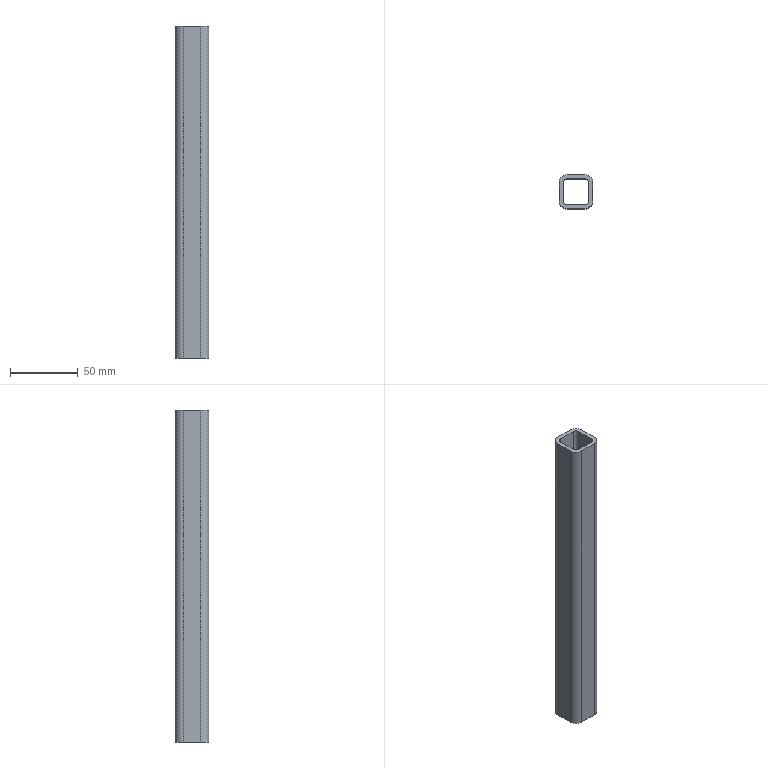Part | STEP file | ISO 10799-2 25x25x3 1784906820939 | 1 solid | 18 faces | box 25 x 25 x 245 mm | volume 59002 mm3 | plane 10 | cylinder 8 | commonest cylinder face diameters 6 x4 12 x4
STEP:
#1=CARTESIAN_POINT('',(-6.5,-9.5,245.));
#2=VERTEX_POINT('',#1);
#3=CARTESIAN_POINT('',(6.5,-9.5,245.));
#4=VERTEX_POINT('',#3);
#5=CARTESIAN_POINT('',(3.25,-9.5,245.));
#6=DIRECTION('',(1.,0.,0.));
#7=VECTOR('',#6,10.);
#8=LINE('',#5,#7);
#9=EDGE_CURVE('',#2,#4,#8,.T.);
#10=ORIENTED_EDGE('',*,*,#9,.T.);
#11=CARTESIAN_POINT('',(6.5,-9.5,0.));
#12=VERTEX_POINT('',#11);
#13=CARTESIAN_POINT('',(6.5,-9.5,0.));
#14=DIRECTION('',(0.,0.,1.));
#15=VECTOR('',#14,10.);
#16=LINE('',#13,#15);
#17=EDGE_CURVE('',#12,#4,#16,.T.);
#18=ORIENTED_EDGE('',*,*,#17,.F.);
#19=CARTESIAN_POINT('',(-6.5,-9.5,0.));
#20=VERTEX_POINT('',#19);
#21=CARTESIAN_POINT('',(3.25,-9.5,0.));
#22=DIRECTION('',(1.,0.,0.));
#23=VECTOR('',#22,10.);
#24=LINE('',#21,#23);
#25=EDGE_CURVE('',#20,#12,#24,.T.);
#26=ORIENTED_EDGE('',*,*,#25,.F.);
#27=CARTESIAN_POINT('',(-6.5,-9.5,0.));
#28=DIRECTION('',(0.,0.,1.));
#29=VECTOR('',#28,10.);
#30=LINE('',#27,#29);
#31=EDGE_CURVE('',#20,#2,#30,.T.);
#32=ORIENTED_EDGE('',*,*,#31,.T.);
#33=EDGE_LOOP('',(#10,#18,#26,#32));
#34=FACE_OUTER_BOUND('',#33,.T.);
#35=CARTESIAN_POINT('',(6.5,-9.5,0.));
#36=DIRECTION('',(0.,-1.,0.));
#37=DIRECTION('',(0.,0.,-1.));
#38=AXIS2_PLACEMENT_3D('',#35,#36,#37);
#39=PLANE('',#38);
#40=ADVANCED_FACE('',(#34),#39,.F.);
#41=CARTESIAN_POINT('',(9.5,-6.5,245.));
#42=VERTEX_POINT('',#41);
#43=CARTESIAN_POINT('',(6.5,-6.5,245.));
#44=DIRECTION('',(0.,0.,1.));
#45=DIRECTION('',(0.,1.,0.));
#46=AXIS2_PLACEMENT_3D('',#43,#44,#45);
#47=CIRCLE('',#46,3.);
#48=EDGE_CURVE('',#4,#42,#47,.T.);
#49=ORIENTED_EDGE('',*,*,#48,.T.);
#50=CARTESIAN_POINT('',(9.5,-6.5,0.));
#51=VERTEX_POINT('',#50);
#52=CARTESIAN_POINT('',(9.5,-6.5,0.));
#53=DIRECTION('',(0.,0.,1.));
#54=VECTOR('',#53,10.);
#55=LINE('',#52,#54);
#56=EDGE_CURVE('',#51,#42,#55,.T.);
#57=ORIENTED_EDGE('',*,*,#56,.F.);
#58=CARTESIAN_POINT('',(6.5,-6.5,0.));
#59=DIRECTION('',(0.,0.,1.));
#60=DIRECTION('',(0.,1.,0.));
#61=AXIS2_PLACEMENT_3D('',#58,#59,#60);
#62=CIRCLE('',#61,3.);
#63=EDGE_CURVE('',#12,#51,#62,.T.);
#64=ORIENTED_EDGE('',*,*,#63,.F.);
#65=ORIENTED_EDGE('',*,*,#17,.T.);
#66=EDGE_LOOP('',(#49,#57,#64,#65));
#67=FACE_OUTER_BOUND('',#66,.T.);
#68=CARTESIAN_POINT('',(6.5,-6.5,0.));
#69=DIRECTION('',(0.,0.,1.));
#70=DIRECTION('',(0.,1.,0.));
#71=AXIS2_PLACEMENT_3D('',#68,#69,#70);
#72=CYLINDRICAL_SURFACE('',#71,3.);
#73=ADVANCED_FACE('',(#67),#72,.F.);
#74=CARTESIAN_POINT('',(9.5,6.5,245.));
#75=VERTEX_POINT('',#74);
#76=CARTESIAN_POINT('',(9.5,3.25,245.));
#77=DIRECTION('',(0.,1.,0.));
#78=VECTOR('',#77,10.);
#79=LINE('',#76,#78);
#80=EDGE_CURVE('',#42,#75,#79,.T.);
#81=ORIENTED_EDGE('',*,*,#80,.T.);
#82=CARTESIAN_POINT('',(9.5,6.5,0.));
#83=VERTEX_POINT('',#82);
#84=CARTESIAN_POINT('',(9.5,6.5,0.));
#85=DIRECTION('',(0.,0.,1.));
#86=VECTOR('',#85,10.);
#87=LINE('',#84,#86);
#88=EDGE_CURVE('',#83,#75,#87,.T.);
#89=ORIENTED_EDGE('',*,*,#88,.F.);
#90=CARTESIAN_POINT('',(9.5,3.25,0.));
#91=DIRECTION('',(0.,1.,0.));
#92=VECTOR('',#91,10.);
#93=LINE('',#90,#92);
#94=EDGE_CURVE('',#51,#83,#93,.T.);
#95=ORIENTED_EDGE('',*,*,#94,.F.);
#96=ORIENTED_EDGE('',*,*,#56,.T.);
#97=EDGE_LOOP('',(#81,#89,#95,#96));
#98=FACE_OUTER_BOUND('',#97,.T.);
#99=CARTESIAN_POINT('',(9.5,6.5,0.));
#100=DIRECTION('',(1.,0.,0.));
#101=DIRECTION('',(0.,0.,-1.));
#102=AXIS2_PLACEMENT_3D('',#99,#100,#101);
#103=PLANE('',#102);
#104=ADVANCED_FACE('',(#98),#103,.F.);
#105=CARTESIAN_POINT('',(6.5,9.5,245.));
#106=VERTEX_POINT('',#105);
#107=CARTESIAN_POINT('',(6.5,6.5,245.));
#108=DIRECTION('',(0.,0.,1.));
#109=DIRECTION('',(-1.,0.,0.));
#110=AXIS2_PLACEMENT_3D('',#107,#108,#109);
#111=CIRCLE('',#110,3.);
#112=EDGE_CURVE('',#75,#106,#111,.T.);
#113=ORIENTED_EDGE('',*,*,#112,.T.);
#114=CARTESIAN_POINT('',(6.5,9.5,0.));
#115=VERTEX_POINT('',#114);
#116=CARTESIAN_POINT('',(6.5,9.5,0.));
#117=DIRECTION('',(0.,0.,1.));
#118=VECTOR('',#117,10.);
#119=LINE('',#116,#118);
#120=EDGE_CURVE('',#115,#106,#119,.T.);
#121=ORIENTED_EDGE('',*,*,#120,.F.);
#122=CARTESIAN_POINT('',(6.5,6.5,0.));
#123=DIRECTION('',(0.,0.,1.));
#124=DIRECTION('',(-1.,0.,0.));
#125=AXIS2_PLACEMENT_3D('',#122,#123,#124);
#126=CIRCLE('',#125,3.);
#127=EDGE_CURVE('',#83,#115,#126,.T.);
#128=ORIENTED_EDGE('',*,*,#127,.F.);
#129=ORIENTED_EDGE('',*,*,#88,.T.);
#130=EDGE_LOOP('',(#113,#121,#128,#129));
#131=FACE_OUTER_BOUND('',#130,.T.);
#132=CARTESIAN_POINT('',(6.5,6.5,0.));
#133=DIRECTION('',(0.,0.,1.));
#134=DIRECTION('',(-1.,0.,0.));
#135=AXIS2_PLACEMENT_3D('',#132,#133,#134);
#136=CYLINDRICAL_SURFACE('',#135,3.);
#137=ADVANCED_FACE('',(#131),#136,.F.);
#138=CARTESIAN_POINT('',(12.5,6.5,245.));
#139=VERTEX_POINT('',#138);
#140=CARTESIAN_POINT('',(12.5,-6.5,245.));
#141=VERTEX_POINT('',#140);
#142=CARTESIAN_POINT('',(12.5,3.25,245.));
#143=DIRECTION('',(0.,-1.,0.));
#144=VECTOR('',#143,10.);
#145=LINE('',#142,#144);
#146=EDGE_CURVE('',#139,#141,#145,.T.);
#147=ORIENTED_EDGE('',*,*,#146,.T.);
#148=CARTESIAN_POINT('',(12.5,-6.5,0.));
#149=VERTEX_POINT('',#148);
#150=CARTESIAN_POINT('',(12.5,-6.5,0.));
#151=DIRECTION('',(0.,0.,1.));
#152=VECTOR('',#151,10.);
#153=LINE('',#150,#152);
#154=EDGE_CURVE('',#149,#141,#153,.T.);
#155=ORIENTED_EDGE('',*,*,#154,.F.);
#156=CARTESIAN_POINT('',(12.5,6.5,0.));
#157=VERTEX_POINT('',#156);
#158=CARTESIAN_POINT('',(12.5,3.25,0.));
#159=DIRECTION('',(0.,-1.,0.));
#160=VECTOR('',#159,10.);
#161=LINE('',#158,#160);
#162=EDGE_CURVE('',#157,#149,#161,.T.);
#163=ORIENTED_EDGE('',*,*,#162,.F.);
#164=CARTESIAN_POINT('',(12.5,6.5,0.));
#165=DIRECTION('',(0.,0.,1.));
#166=VECTOR('',#165,10.);
#167=LINE('',#164,#166);
#168=EDGE_CURVE('',#157,#139,#167,.T.);
#169=ORIENTED_EDGE('',*,*,#168,.T.);
#170=EDGE_LOOP('',(#147,#155,#163,#169));
#171=FACE_OUTER_BOUND('',#170,.T.);
#172=CARTESIAN_POINT('',(12.5,6.5,0.));
#173=DIRECTION('',(1.,0.,0.));
#174=DIRECTION('',(0.,0.,-1.));
#175=AXIS2_PLACEMENT_3D('',#172,#173,#174);
#176=PLANE('',#175);
#177=ADVANCED_FACE('',(#171),#176,.T.);
#178=CARTESIAN_POINT('',(6.5,-12.5,245.));
#179=VERTEX_POINT('',#178);
#180=CARTESIAN_POINT('',(6.5,-6.5,245.));
#181=DIRECTION('',(0.,0.,-1.));
#182=DIRECTION('',(0.,1.,0.));
#183=AXIS2_PLACEMENT_3D('',#180,#181,#182);
#184=CIRCLE('',#183,6.);
#185=EDGE_CURVE('',#141,#179,#184,.T.);
#186=ORIENTED_EDGE('',*,*,#185,.T.);
#187=CARTESIAN_POINT('',(6.5,-12.5,0.));
#188=VERTEX_POINT('',#187);
#189=CARTESIAN_POINT('',(6.5,-12.5,0.));
#190=DIRECTION('',(0.,0.,1.));
#191=VECTOR('',#190,10.);
#192=LINE('',#189,#191);
#193=EDGE_CURVE('',#188,#179,#192,.T.);
#194=ORIENTED_EDGE('',*,*,#193,.F.);
#195=CARTESIAN_POINT('',(6.5,-6.5,0.));
#196=DIRECTION('',(0.,0.,-1.));
#197=DIRECTION('',(0.,1.,0.));
#198=AXIS2_PLACEMENT_3D('',#195,#196,#197);
#199=CIRCLE('',#198,6.);
#200=EDGE_CURVE('',#149,#188,#199,.T.);
#201=ORIENTED_EDGE('',*,*,#200,.F.);
#202=ORIENTED_EDGE('',*,*,#154,.T.);
#203=EDGE_LOOP('',(#186,#194,#201,#202));
#204=FACE_OUTER_BOUND('',#203,.T.);
#205=CARTESIAN_POINT('',(6.5,-6.5,0.));
#206=DIRECTION('',(0.,0.,1.));
#207=DIRECTION('',(0.,1.,0.));
#208=AXIS2_PLACEMENT_3D('',#205,#206,#207);
#209=CYLINDRICAL_SURFACE('',#208,6.);
#210=ADVANCED_FACE('',(#204),#209,.T.);
#211=CARTESIAN_POINT('',(-6.5,-12.5,245.));
#212=VERTEX_POINT('',#211);
#213=CARTESIAN_POINT('',(3.25,-12.5,245.));
#214=DIRECTION('',(-1.,0.,0.));
#215=VECTOR('',#214,10.);
#216=LINE('',#213,#215);
#217=EDGE_CURVE('',#179,#212,#216,.T.);
#218=ORIENTED_EDGE('',*,*,#217,.T.);
#219=CARTESIAN_POINT('',(-6.5,-12.5,0.));
#220=VERTEX_POINT('',#219);
#221=CARTESIAN_POINT('',(-6.5,-12.5,0.));
#222=DIRECTION('',(0.,0.,1.));
#223=VECTOR('',#222,10.);
#224=LINE('',#221,#223);
#225=EDGE_CURVE('',#220,#212,#224,.T.);
#226=ORIENTED_EDGE('',*,*,#225,.F.);
#227=CARTESIAN_POINT('',(3.25,-12.5,0.));
#228=DIRECTION('',(-1.,0.,0.));
#229=VECTOR('',#228,10.);
#230=LINE('',#227,#229);
#231=EDGE_CURVE('',#188,#220,#230,.T.);
#232=ORIENTED_EDGE('',*,*,#231,.F.);
#233=ORIENTED_EDGE('',*,*,#193,.T.);
#234=EDGE_LOOP('',(#218,#226,#232,#233));
#235=FACE_OUTER_BOUND('',#234,.T.);
#236=CARTESIAN_POINT('',(6.5,-12.5,0.));
#237=DIRECTION('',(0.,-1.,0.));
#238=DIRECTION('',(0.,0.,-1.));
#239=AXIS2_PLACEMENT_3D('',#236,#237,#238);
#240=PLANE('',#239);
#241=ADVANCED_FACE('',(#235),#240,.T.);
#242=CARTESIAN_POINT('',(-12.5,-6.5,245.));
#243=VERTEX_POINT('',#242);
#244=CARTESIAN_POINT('',(-6.5,-6.5,245.));
#245=DIRECTION('',(0.,0.,-1.));
#246=DIRECTION('',(1.,0.,0.));
#247=AXIS2_PLACEMENT_3D('',#244,#245,#246);
#248=CIRCLE('',#247,6.);
#249=EDGE_CURVE('',#212,#243,#248,.T.);
#250=ORIENTED_EDGE('',*,*,#249,.T.);
#251=CARTESIAN_POINT('',(-12.5,-6.5,0.));
#252=VERTEX_POINT('',#251);
#253=CARTESIAN_POINT('',(-12.5,-6.5,0.));
#254=DIRECTION('',(0.,0.,1.));
#255=VECTOR('',#254,10.);
#256=LINE('',#253,#255);
#257=EDGE_CURVE('',#252,#243,#256,.T.);
#258=ORIENTED_EDGE('',*,*,#257,.F.);
#259=CARTESIAN_POINT('',(-6.5,-6.5,0.));
#260=DIRECTION('',(0.,0.,-1.));
#261=DIRECTION('',(1.,0.,0.));
#262=AXIS2_PLACEMENT_3D('',#259,#260,#261);
#263=CIRCLE('',#262,6.);
#264=EDGE_CURVE('',#220,#252,#263,.T.);
#265=ORIENTED_EDGE('',*,*,#264,.F.);
#266=ORIENTED_EDGE('',*,*,#225,.T.);
#267=EDGE_LOOP('',(#250,#258,#265,#266));
#268=FACE_OUTER_BOUND('',#267,.T.);
#269=CARTESIAN_POINT('',(-6.5,-6.5,0.));
#270=DIRECTION('',(0.,0.,1.));
#271=DIRECTION('',(1.,0.,0.));
#272=AXIS2_PLACEMENT_3D('',#269,#270,#271);
#273=CYLINDRICAL_SURFACE('',#272,6.);
#274=ADVANCED_FACE('',(#268),#273,.T.);
#275=CARTESIAN_POINT('',(-6.5,9.5,245.));
#276=VERTEX_POINT('',#275);
#277=CARTESIAN_POINT('',(-3.25,9.5,245.));
#278=DIRECTION('',(-1.,0.,0.));
#279=VECTOR('',#278,10.);
#280=LINE('',#277,#279);
#281=EDGE_CURVE('',#106,#276,#280,.T.);
#282=ORIENTED_EDGE('',*,*,#281,.T.);
#283=CARTESIAN_POINT('',(-6.5,9.5,0.));
#284=VERTEX_POINT('',#283);
#285=CARTESIAN_POINT('',(-6.5,9.5,0.));
#286=DIRECTION('',(0.,0.,1.));
#287=VECTOR('',#286,10.);
#288=LINE('',#285,#287);
#289=EDGE_CURVE('',#284,#276,#288,.T.);
#290=ORIENTED_EDGE('',*,*,#289,.F.);
#291=CARTESIAN_POINT('',(-3.25,9.5,0.));
#292=DIRECTION('',(-1.,0.,0.));
#293=VECTOR('',#292,10.);
#294=LINE('',#291,#293);
#295=EDGE_CURVE('',#115,#284,#294,.T.);
#296=ORIENTED_EDGE('',*,*,#295,.F.);
#297=ORIENTED_EDGE('',*,*,#120,.T.);
#298=EDGE_LOOP('',(#282,#290,#296,#297));
#299=FACE_OUTER_BOUND('',#298,.T.);
#300=CARTESIAN_POINT('',(-6.5,9.5,0.));
#301=DIRECTION('',(0.,1.,0.));
#302=DIRECTION('',(0.,0.,1.));
#303=AXIS2_PLACEMENT_3D('',#300,#301,#302);
#304=PLANE('',#303);
#305=ADVANCED_FACE('',(#299),#304,.F.);
#306=CARTESIAN_POINT('',(-9.5,-6.5,245.));
#307=VERTEX_POINT('',#306);
#308=CARTESIAN_POINT('',(-6.5,-6.5,245.));
#309=DIRECTION('',(0.,0.,1.));
#310=DIRECTION('',(1.,0.,0.));
#311=AXIS2_PLACEMENT_3D('',#308,#309,#310);
#312=CIRCLE('',#311,3.);
#313=EDGE_CURVE('',#307,#2,#312,.T.);
#314=ORIENTED_EDGE('',*,*,#313,.T.);
#315=ORIENTED_EDGE('',*,*,#31,.F.);
#316=CARTESIAN_POINT('',(-9.5,-6.5,0.));
#317=VERTEX_POINT('',#316);
#318=CARTESIAN_POINT('',(-6.5,-6.5,0.));
#319=DIRECTION('',(0.,0.,1.));
#320=DIRECTION('',(1.,0.,0.));
#321=AXIS2_PLACEMENT_3D('',#318,#319,#320);
#322=CIRCLE('',#321,3.);
#323=EDGE_CURVE('',#317,#20,#322,.T.);
#324=ORIENTED_EDGE('',*,*,#323,.F.);
#325=CARTESIAN_POINT('',(-9.5,-6.5,0.));
#326=DIRECTION('',(0.,0.,1.));
#327=VECTOR('',#326,10.);
#328=LINE('',#325,#327);
#329=EDGE_CURVE('',#317,#307,#328,.T.);
#330=ORIENTED_EDGE('',*,*,#329,.T.);
#331=EDGE_LOOP('',(#314,#315,#324,#330));
#332=FACE_OUTER_BOUND('',#331,.T.);
#333=CARTESIAN_POINT('',(-6.5,-6.5,0.));
#334=DIRECTION('',(0.,0.,1.));
#335=DIRECTION('',(1.,0.,0.));
#336=AXIS2_PLACEMENT_3D('',#333,#334,#335);
#337=CYLINDRICAL_SURFACE('',#336,3.);
#338=ADVANCED_FACE('',(#332),#337,.F.);
#339=CARTESIAN_POINT('',(-9.5,6.5,245.));
#340=VERTEX_POINT('',#339);
#341=CARTESIAN_POINT('',(-9.5,-3.25,245.));
#342=DIRECTION('',(0.,-1.,0.));
#343=VECTOR('',#342,10.);
#344=LINE('',#341,#343);
#345=EDGE_CURVE('',#340,#307,#344,.T.);
#346=ORIENTED_EDGE('',*,*,#345,.T.);
#347=ORIENTED_EDGE('',*,*,#329,.F.);
#348=CARTESIAN_POINT('',(-9.5,6.5,0.));
#349=VERTEX_POINT('',#348);
#350=CARTESIAN_POINT('',(-9.5,-3.25,0.));
#351=DIRECTION('',(0.,-1.,0.));
#352=VECTOR('',#351,10.);
#353=LINE('',#350,#352);
#354=EDGE_CURVE('',#349,#317,#353,.T.);
#355=ORIENTED_EDGE('',*,*,#354,.F.);
#356=CARTESIAN_POINT('',(-9.5,6.5,0.));
#357=DIRECTION('',(0.,0.,1.));
#358=VECTOR('',#357,10.);
#359=LINE('',#356,#358);
#360=EDGE_CURVE('',#349,#340,#359,.T.);
#361=ORIENTED_EDGE('',*,*,#360,.T.);
#362=EDGE_LOOP('',(#346,#347,#355,#361));
#363=FACE_OUTER_BOUND('',#362,.T.);
#364=CARTESIAN_POINT('',(-9.5,-6.5,0.));
#365=DIRECTION('',(-1.,0.,0.));
#366=DIRECTION('',(0.,0.,1.));
#367=AXIS2_PLACEMENT_3D('',#364,#365,#366);
#368=PLANE('',#367);
#369=ADVANCED_FACE('',(#363),#368,.F.);
#370=CARTESIAN_POINT('',(-6.5,6.5,245.));
#371=DIRECTION('',(0.,0.,1.));
#372=DIRECTION('',(0.,-1.,0.));
#373=AXIS2_PLACEMENT_3D('',#370,#371,#372);
#374=CIRCLE('',#373,3.);
#375=EDGE_CURVE('',#276,#340,#374,.T.);
#376=ORIENTED_EDGE('',*,*,#375,.T.);
#377=ORIENTED_EDGE('',*,*,#360,.F.);
#378=CARTESIAN_POINT('',(-6.5,6.5,0.));
#379=DIRECTION('',(0.,0.,1.));
#380=DIRECTION('',(0.,-1.,0.));
#381=AXIS2_PLACEMENT_3D('',#378,#379,#380);
#382=CIRCLE('',#381,3.);
#383=EDGE_CURVE('',#284,#349,#382,.T.);
#384=ORIENTED_EDGE('',*,*,#383,.F.);
#385=ORIENTED_EDGE('',*,*,#289,.T.);
#386=EDGE_LOOP('',(#376,#377,#384,#385));
#387=FACE_OUTER_BOUND('',#386,.T.);
#388=CARTESIAN_POINT('',(-6.5,6.5,0.));
#389=DIRECTION('',(0.,0.,1.));
#390=DIRECTION('',(0.,-1.,0.));
#391=AXIS2_PLACEMENT_3D('',#388,#389,#390);
#392=CYLINDRICAL_SURFACE('',#391,3.);
#393=ADVANCED_FACE('',(#387),#392,.F.);
#394=CARTESIAN_POINT('',(-12.5,6.5,245.));
#395=VERTEX_POINT('',#394);
#396=CARTESIAN_POINT('',(-12.5,-3.25,245.));
#397=DIRECTION('',(0.,1.,0.));
#398=VECTOR('',#397,10.);
#399=LINE('',#396,#398);
#400=EDGE_CURVE('',#243,#395,#399,.T.);
#401=ORIENTED_EDGE('',*,*,#400,.T.);
#402=CARTESIAN_POINT('',(-12.5,6.5,0.));
#403=VERTEX_POINT('',#402);
#404=CARTESIAN_POINT('',(-12.5,6.5,0.));
#405=DIRECTION('',(0.,0.,1.));
#406=VECTOR('',#405,10.);
#407=LINE('',#404,#406);
#408=EDGE_CURVE('',#403,#395,#407,.T.);
#409=ORIENTED_EDGE('',*,*,#408,.F.);
#410=CARTESIAN_POINT('',(-12.5,-3.25,0.));
#411=DIRECTION('',(0.,1.,0.));
#412=VECTOR('',#411,10.);
#413=LINE('',#410,#412);
#414=EDGE_CURVE('',#252,#403,#413,.T.);
#415=ORIENTED_EDGE('',*,*,#414,.F.);
#416=ORIENTED_EDGE('',*,*,#257,.T.);
#417=EDGE_LOOP('',(#401,#409,#415,#416));
#418=FACE_OUTER_BOUND('',#417,.T.);
#419=CARTESIAN_POINT('',(-12.5,-6.5,0.));
#420=DIRECTION('',(-1.,0.,0.));
#421=DIRECTION('',(0.,0.,1.));
#422=AXIS2_PLACEMENT_3D('',#419,#420,#421);
#423=PLANE('',#422);
#424=ADVANCED_FACE('',(#418),#423,.T.);
#425=CARTESIAN_POINT('',(-6.5,12.5,245.));
#426=VERTEX_POINT('',#425);
#427=CARTESIAN_POINT('',(-6.5,6.5,245.));
#428=DIRECTION('',(0.,0.,-1.));
#429=DIRECTION('',(0.,-1.,0.));
#430=AXIS2_PLACEMENT_3D('',#427,#428,#429);
#431=CIRCLE('',#430,6.);
#432=EDGE_CURVE('',#395,#426,#431,.T.);
#433=ORIENTED_EDGE('',*,*,#432,.T.);
#434=CARTESIAN_POINT('',(-6.5,12.5,0.));
#435=VERTEX_POINT('',#434);
#436=CARTESIAN_POINT('',(-6.5,12.5,0.));
#437=DIRECTION('',(0.,0.,1.));
#438=VECTOR('',#437,10.);
#439=LINE('',#436,#438);
#440=EDGE_CURVE('',#435,#426,#439,.T.);
#441=ORIENTED_EDGE('',*,*,#440,.F.);
#442=CARTESIAN_POINT('',(-6.5,6.5,0.));
#443=DIRECTION('',(0.,0.,-1.));
#444=DIRECTION('',(0.,-1.,0.));
#445=AXIS2_PLACEMENT_3D('',#442,#443,#444);
#446=CIRCLE('',#445,6.);
#447=EDGE_CURVE('',#403,#435,#446,.T.);
#448=ORIENTED_EDGE('',*,*,#447,.F.);
#449=ORIENTED_EDGE('',*,*,#408,.T.);
#450=EDGE_LOOP('',(#433,#441,#448,#449));
#451=FACE_OUTER_BOUND('',#450,.T.);
#452=CARTESIAN_POINT('',(-6.5,6.5,0.));
#453=DIRECTION('',(0.,0.,1.));
#454=DIRECTION('',(0.,-1.,0.));
#455=AXIS2_PLACEMENT_3D('',#452,#453,#454);
#456=CYLINDRICAL_SURFACE('',#455,6.);
#457=ADVANCED_FACE('',(#451),#456,.T.);
#458=CARTESIAN_POINT('',(6.5,12.5,245.));
#459=VERTEX_POINT('',#458);
#460=CARTESIAN_POINT('',(-3.25,12.5,245.));
#461=DIRECTION('',(1.,0.,0.));
#462=VECTOR('',#461,10.);
#463=LINE('',#460,#462);
#464=EDGE_CURVE('',#426,#459,#463,.T.);
#465=ORIENTED_EDGE('',*,*,#464,.T.);
#466=CARTESIAN_POINT('',(6.5,12.5,0.));
#467=VERTEX_POINT('',#466);
#468=CARTESIAN_POINT('',(6.5,12.5,0.));
#469=DIRECTION('',(0.,0.,1.));
#470=VECTOR('',#469,10.);
#471=LINE('',#468,#470);
#472=EDGE_CURVE('',#467,#459,#471,.T.);
#473=ORIENTED_EDGE('',*,*,#472,.F.);
#474=CARTESIAN_POINT('',(-3.25,12.5,0.));
#475=DIRECTION('',(1.,0.,0.));
#476=VECTOR('',#475,10.);
#477=LINE('',#474,#476);
#478=EDGE_CURVE('',#435,#467,#477,.T.);
#479=ORIENTED_EDGE('',*,*,#478,.F.);
#480=ORIENTED_EDGE('',*,*,#440,.T.);
#481=EDGE_LOOP('',(#465,#473,#479,#480));
#482=FACE_OUTER_BOUND('',#481,.T.);
#483=CARTESIAN_POINT('',(-6.5,12.5,0.));
#484=DIRECTION('',(0.,1.,0.));
#485=DIRECTION('',(0.,0.,1.));
#486=AXIS2_PLACEMENT_3D('',#483,#484,#485);
#487=PLANE('',#486);
#488=ADVANCED_FACE('',(#482),#487,.T.);
#489=CARTESIAN_POINT('',(6.5,6.5,245.));
#490=DIRECTION('',(0.,0.,-1.));
#491=DIRECTION('',(-1.,0.,0.));
#492=AXIS2_PLACEMENT_3D('',#489,#490,#491);
#493=CIRCLE('',#492,6.);
#494=EDGE_CURVE('',#459,#139,#493,.T.);
#495=ORIENTED_EDGE('',*,*,#494,.T.);
#496=ORIENTED_EDGE('',*,*,#168,.F.);
#497=CARTESIAN_POINT('',(6.5,6.5,0.));
#498=DIRECTION('',(0.,0.,-1.));
#499=DIRECTION('',(-1.,0.,0.));
#500=AXIS2_PLACEMENT_3D('',#497,#498,#499);
#501=CIRCLE('',#500,6.);
#502=EDGE_CURVE('',#467,#157,#501,.T.);
#503=ORIENTED_EDGE('',*,*,#502,.F.);
#504=ORIENTED_EDGE('',*,*,#472,.T.);
#505=EDGE_LOOP('',(#495,#496,#503,#504));
#506=FACE_OUTER_BOUND('',#505,.T.);
#507=CARTESIAN_POINT('',(6.5,6.5,0.));
#508=DIRECTION('',(0.,0.,1.));
#509=DIRECTION('',(-1.,0.,0.));
#510=AXIS2_PLACEMENT_3D('',#507,#508,#509);
#511=CYLINDRICAL_SURFACE('',#510,6.);
#512=ADVANCED_FACE('',(#506),#511,.T.);
#513=ORIENTED_EDGE('',*,*,#414,.T.);
#514=ORIENTED_EDGE('',*,*,#447,.T.);
#515=ORIENTED_EDGE('',*,*,#478,.T.);
#516=ORIENTED_EDGE('',*,*,#502,.T.);
#517=ORIENTED_EDGE('',*,*,#162,.T.);
#518=ORIENTED_EDGE('',*,*,#200,.T.);
#519=ORIENTED_EDGE('',*,*,#231,.T.);
#520=ORIENTED_EDGE('',*,*,#264,.T.);
#521=EDGE_LOOP('',(#513,#514,#515,#516,#517,#518,#519,#520));
#522=FACE_OUTER_BOUND('',#521,.T.);
#523=ORIENTED_EDGE('',*,*,#295,.T.);
#524=ORIENTED_EDGE('',*,*,#383,.T.);
#525=ORIENTED_EDGE('',*,*,#354,.T.);
#526=ORIENTED_EDGE('',*,*,#323,.T.);
#527=ORIENTED_EDGE('',*,*,#25,.T.);
#528=ORIENTED_EDGE('',*,*,#63,.T.);
#529=ORIENTED_EDGE('',*,*,#94,.T.);
#530=ORIENTED_EDGE('',*,*,#127,.T.);
#531=EDGE_LOOP('',(#523,#524,#525,#526,#527,#528,#529,#530));
#532=FACE_BOUND('',#531,.T.);
#533=CARTESIAN_POINT('',(0.,0.,0.));
#534=DIRECTION('',(0.,0.,1.));
#535=DIRECTION('',(1.,0.,0.));
#536=AXIS2_PLACEMENT_3D('',#533,#534,#535);
#537=PLANE('',#536);
#538=ADVANCED_FACE('',(#522,#532),#537,.F.);
#539=ORIENTED_EDGE('',*,*,#400,.F.);
#540=ORIENTED_EDGE('',*,*,#249,.F.);
#541=ORIENTED_EDGE('',*,*,#217,.F.);
#542=ORIENTED_EDGE('',*,*,#185,.F.);
#543=ORIENTED_EDGE('',*,*,#146,.F.);
#544=ORIENTED_EDGE('',*,*,#494,.F.);
#545=ORIENTED_EDGE('',*,*,#464,.F.);
#546=ORIENTED_EDGE('',*,*,#432,.F.);
#547=EDGE_LOOP('',(#539,#540,#541,#542,#543,#544,#545,#546));
#548=FACE_OUTER_BOUND('',#547,.T.);
#549=ORIENTED_EDGE('',*,*,#281,.F.);
#550=ORIENTED_EDGE('',*,*,#112,.F.);
#551=ORIENTED_EDGE('',*,*,#80,.F.);
#552=ORIENTED_EDGE('',*,*,#48,.F.);
#553=ORIENTED_EDGE('',*,*,#9,.F.);
#554=ORIENTED_EDGE('',*,*,#313,.F.);
#555=ORIENTED_EDGE('',*,*,#345,.F.);
#556=ORIENTED_EDGE('',*,*,#375,.F.);
#557=EDGE_LOOP('',(#549,#550,#551,#552,#553,#554,#555,#556));
#558=FACE_BOUND('',#557,.T.);
#559=CARTESIAN_POINT('',(0.,0.,245.));
#560=DIRECTION('',(0.,0.,1.));
#561=DIRECTION('',(1.,0.,0.));
#562=AXIS2_PLACEMENT_3D('',#559,#560,#561);
#563=PLANE('',#562);
#564=ADVANCED_FACE('',(#548,#558),#563,.T.);
#565=CLOSED_SHELL('',(#40,#73,#104,#137,#177,#210,#241,#274,#305,#338,#369,#393,#424,#457,#488,#512,#538,#564));
#566=MANIFOLD_SOLID_BREP('',#565);
#567=(LENGTH_UNIT()NAMED_UNIT(*)SI_UNIT(.MILLI.,.METRE.));
#568=UNCERTAINTY_MEASURE_WITH_UNIT(LENGTH_MEASURE(0.01),#567,'','');
#569=(NAMED_UNIT(*)PLANE_ANGLE_UNIT()SI_UNIT($,.RADIAN.));
#570=(NAMED_UNIT(*)SI_UNIT($,.STERADIAN.)SOLID_ANGLE_UNIT());
#571=(GEOMETRIC_REPRESENTATION_CONTEXT(3)GLOBAL_UNCERTAINTY_ASSIGNED_CONTEXT((#568))GLOBAL_UNIT_ASSIGNED_CONTEXT((#567,#569,#570))REPRESENTATION_CONTEXT('',''));
#572=ADVANCED_BREP_SHAPE_REPRESENTATION('',(#566),#571);